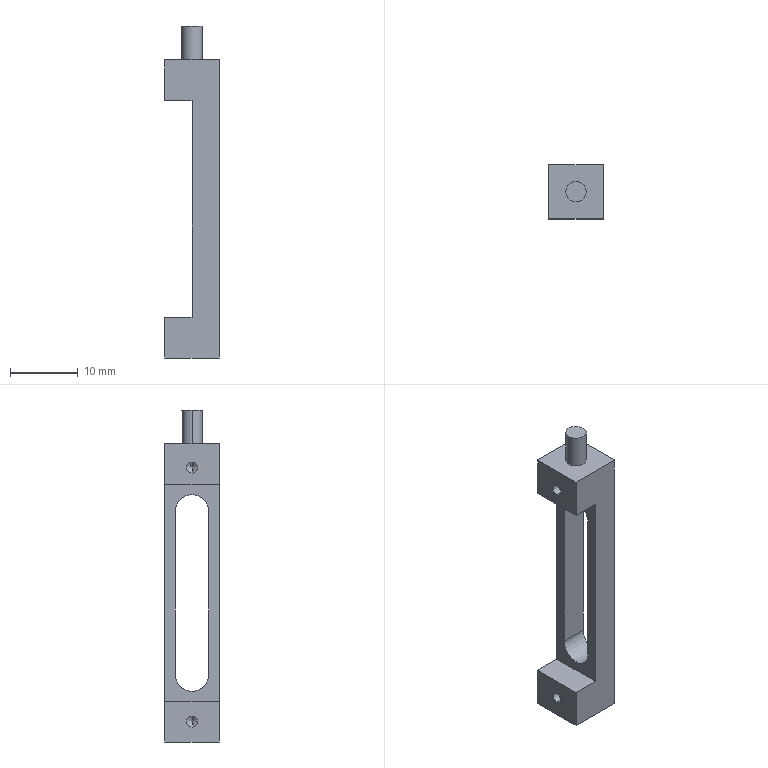Part | STEP file | 06-01-16 light source mounting plate | 1 solid | 25 faces | box 8 x 8 x 49 mm | volume 1247 mm3 | plane 13 | cylinder 8 | cone 4 | commonest cylinder face diameters 1.6 x4 3 x2 5 x2
STEP:
#1=CARTESIAN_POINT('',(1.2,0.,39.7));
#2=VERTEX_POINT('',#1);
#3=CARTESIAN_POINT('',(1.2,0.,41.3));
#4=VERTEX_POINT('',#3);
#5=CARTESIAN_POINT('',(1.2,0.,40.5));
#6=DIRECTION('',(-1.,0.,0.));
#7=DIRECTION('',(0.,0.,1.));
#8=AXIS2_PLACEMENT_3D('',#5,#6,#7);
#9=CIRCLE('',#8,0.8);
#10=EDGE_CURVE('',#2,#4,#9,.T.);
#11=ORIENTED_EDGE('',*,*,#10,.F.);
#12=CARTESIAN_POINT('',(-4.,0.,39.7));
#13=VERTEX_POINT('',#12);
#14=CARTESIAN_POINT('',(-4.,0.,39.7));
#15=DIRECTION('',(-1.,0.,0.));
#16=VECTOR('',#15,1000.);
#17=LINE('',#14,#16);
#18=EDGE_CURVE('',#2,#13,#17,.T.);
#19=ORIENTED_EDGE('',*,*,#18,.T.);
#20=CARTESIAN_POINT('',(-4.,0.,41.3));
#21=VERTEX_POINT('',#20);
#22=CARTESIAN_POINT('',(-4.,0.,40.5));
#23=DIRECTION('',(-1.,0.,0.));
#24=DIRECTION('',(0.,0.,1.));
#25=AXIS2_PLACEMENT_3D('',#22,#23,#24);
#26=CIRCLE('',#25,0.8);
#27=EDGE_CURVE('',#13,#21,#26,.T.);
#28=ORIENTED_EDGE('',*,*,#27,.T.);
#29=CARTESIAN_POINT('',(-4.,0.,41.3));
#30=DIRECTION('',(-1.,0.,0.));
#31=VECTOR('',#30,1000.);
#32=LINE('',#29,#31);
#33=EDGE_CURVE('',#4,#21,#32,.T.);
#34=ORIENTED_EDGE('',*,*,#33,.F.);
#35=EDGE_LOOP('',(#11,#19,#28,#34));
#36=FACE_OUTER_BOUND('',#35,.T.);
#37=CARTESIAN_POINT('',(-4.,0.,40.5));
#38=DIRECTION('',(-1.,0.,0.));
#39=DIRECTION('',(0.,0.,1.));
#40=AXIS2_PLACEMENT_3D('',#37,#38,#39);
#41=CYLINDRICAL_SURFACE('',#40,0.8);
#42=ADVANCED_FACE('',(#36),#41,.F.);
#43=CARTESIAN_POINT('',(1.681,0.,40.5));
#44=VERTEX_POINT('',#43);
#45=CARTESIAN_POINT('',(1.2,0.,41.3));
#46=DIRECTION('',(-0.515,0.,0.8572));
#47=VECTOR('',#46,1000.);
#48=LINE('',#45,#47);
#49=EDGE_CURVE('',#44,#4,#48,.T.);
#50=ORIENTED_EDGE('',*,*,#49,.F.);
#51=CARTESIAN_POINT('',(1.2,0.,39.7));
#52=DIRECTION('',(-0.515,0.,-0.8572));
#53=VECTOR('',#52,1000.);
#54=LINE('',#51,#53);
#55=EDGE_CURVE('',#44,#2,#54,.T.);
#56=ORIENTED_EDGE('',*,*,#55,.T.);
#57=ORIENTED_EDGE('',*,*,#10,.T.);
#58=EDGE_LOOP('',(#50,#56,#57));
#59=FACE_OUTER_BOUND('',#58,.T.);
#60=CARTESIAN_POINT('',(1.2,0.,40.5));
#61=DIRECTION('',(-1.,0.,0.));
#62=DIRECTION('',(0.,0.,1.));
#63=AXIS2_PLACEMENT_3D('',#60,#61,#62);
#64=CONICAL_SURFACE('',#63,0.8,1.03);
#65=ADVANCED_FACE('',(#59),#64,.F.);
#66=CARTESIAN_POINT('',(1.2,0.,2.2));
#67=VERTEX_POINT('',#66);
#68=CARTESIAN_POINT('',(1.2,0.,3.8));
#69=VERTEX_POINT('',#68);
#70=CARTESIAN_POINT('',(1.2,0.,3.));
#71=DIRECTION('',(-1.,0.,0.));
#72=DIRECTION('',(0.,0.,1.));
#73=AXIS2_PLACEMENT_3D('',#70,#71,#72);
#74=CIRCLE('',#73,0.8);
#75=EDGE_CURVE('',#67,#69,#74,.T.);
#76=ORIENTED_EDGE('',*,*,#75,.F.);
#77=CARTESIAN_POINT('',(-4.,0.,2.2));
#78=VERTEX_POINT('',#77);
#79=CARTESIAN_POINT('',(-4.,0.,2.2));
#80=DIRECTION('',(-1.,0.,0.));
#81=VECTOR('',#80,1000.);
#82=LINE('',#79,#81);
#83=EDGE_CURVE('',#67,#78,#82,.T.);
#84=ORIENTED_EDGE('',*,*,#83,.T.);
#85=CARTESIAN_POINT('',(-4.,0.,3.8));
#86=VERTEX_POINT('',#85);
#87=CARTESIAN_POINT('',(-4.,0.,3.));
#88=DIRECTION('',(-1.,0.,0.));
#89=DIRECTION('',(0.,0.,1.));
#90=AXIS2_PLACEMENT_3D('',#87,#88,#89);
#91=CIRCLE('',#90,0.8);
#92=EDGE_CURVE('',#78,#86,#91,.T.);
#93=ORIENTED_EDGE('',*,*,#92,.T.);
#94=CARTESIAN_POINT('',(-4.,0.,3.8));
#95=DIRECTION('',(-1.,0.,0.));
#96=VECTOR('',#95,1000.);
#97=LINE('',#94,#96);
#98=EDGE_CURVE('',#69,#86,#97,.T.);
#99=ORIENTED_EDGE('',*,*,#98,.F.);
#100=EDGE_LOOP('',(#76,#84,#93,#99));
#101=FACE_OUTER_BOUND('',#100,.T.);
#102=CARTESIAN_POINT('',(-4.,0.,3.));
#103=DIRECTION('',(-1.,0.,0.));
#104=DIRECTION('',(0.,0.,1.));
#105=AXIS2_PLACEMENT_3D('',#102,#103,#104);
#106=CYLINDRICAL_SURFACE('',#105,0.8);
#107=ADVANCED_FACE('',(#101),#106,.F.);
#108=CARTESIAN_POINT('',(1.681,0.,3.));
#109=VERTEX_POINT('',#108);
#110=CARTESIAN_POINT('',(1.2,0.,3.8));
#111=DIRECTION('',(-0.515,0.,0.8572));
#112=VECTOR('',#111,1000.);
#113=LINE('',#110,#112);
#114=EDGE_CURVE('',#109,#69,#113,.T.);
#115=ORIENTED_EDGE('',*,*,#114,.F.);
#116=CARTESIAN_POINT('',(1.2,0.,2.2));
#117=DIRECTION('',(-0.515,0.,-0.8572));
#118=VECTOR('',#117,1000.);
#119=LINE('',#116,#118);
#120=EDGE_CURVE('',#109,#67,#119,.T.);
#121=ORIENTED_EDGE('',*,*,#120,.T.);
#122=ORIENTED_EDGE('',*,*,#75,.T.);
#123=EDGE_LOOP('',(#115,#121,#122));
#124=FACE_OUTER_BOUND('',#123,.T.);
#125=CARTESIAN_POINT('',(1.2,0.,3.));
#126=DIRECTION('',(-1.,0.,0.));
#127=DIRECTION('',(0.,0.,1.));
#128=AXIS2_PLACEMENT_3D('',#125,#126,#127);
#129=CONICAL_SURFACE('',#128,0.8,1.03);
#130=ADVANCED_FACE('',(#124),#129,.F.);
#131=CARTESIAN_POINT('',(1.5,0.,49.));
#132=VERTEX_POINT('',#131);
#133=CARTESIAN_POINT('',(-1.5,0.,49.));
#134=VERTEX_POINT('',#133);
#135=CARTESIAN_POINT('',(0.,0.,49.));
#136=DIRECTION('',(0.,0.,1.));
#137=DIRECTION('',(1.,0.,0.));
#138=AXIS2_PLACEMENT_3D('',#135,#136,#137);
#139=CIRCLE('',#138,1.5);
#140=EDGE_CURVE('',#132,#134,#139,.T.);
#141=ORIENTED_EDGE('',*,*,#140,.F.);
#142=CARTESIAN_POINT('',(1.5,0.,44.));
#143=VERTEX_POINT('',#142);
#144=CARTESIAN_POINT('',(1.5,0.,49.));
#145=DIRECTION('',(0.,0.,-1.));
#146=VECTOR('',#145,1000.);
#147=LINE('',#144,#146);
#148=EDGE_CURVE('',#132,#143,#147,.T.);
#149=ORIENTED_EDGE('',*,*,#148,.T.);
#150=CARTESIAN_POINT('',(-1.5,0.,44.));
#151=VERTEX_POINT('',#150);
#152=CARTESIAN_POINT('',(0.,0.,44.));
#153=DIRECTION('',(0.,0.,1.));
#154=DIRECTION('',(1.,0.,0.));
#155=AXIS2_PLACEMENT_3D('',#152,#153,#154);
#156=CIRCLE('',#155,1.5);
#157=EDGE_CURVE('',#143,#151,#156,.T.);
#158=ORIENTED_EDGE('',*,*,#157,.T.);
#159=CARTESIAN_POINT('',(-1.5,0.,49.));
#160=DIRECTION('',(0.,0.,-1.));
#161=VECTOR('',#160,1000.);
#162=LINE('',#159,#161);
#163=EDGE_CURVE('',#134,#151,#162,.T.);
#164=ORIENTED_EDGE('',*,*,#163,.F.);
#165=EDGE_LOOP('',(#141,#149,#158,#164));
#166=FACE_OUTER_BOUND('',#165,.T.);
#167=CARTESIAN_POINT('',(0.,0.,49.));
#168=DIRECTION('',(0.,0.,-1.));
#169=DIRECTION('',(-1.,0.,0.));
#170=AXIS2_PLACEMENT_3D('',#167,#168,#169);
#171=CYLINDRICAL_SURFACE('',#170,1.5);
#172=ADVANCED_FACE('',(#166),#171,.T.);
#173=CARTESIAN_POINT('',(4.,-4.,44.));
#174=VERTEX_POINT('',#173);
#175=CARTESIAN_POINT('',(4.,4.,44.));
#176=VERTEX_POINT('',#175);
#177=CARTESIAN_POINT('',(4.,4.,44.));
#178=DIRECTION('',(0.,1.,0.));
#179=VECTOR('',#178,1000.);
#180=LINE('',#177,#179);
#181=EDGE_CURVE('',#174,#176,#180,.T.);
#182=ORIENTED_EDGE('',*,*,#181,.T.);
#183=CARTESIAN_POINT('',(-4.,4.,44.));
#184=VERTEX_POINT('',#183);
#185=CARTESIAN_POINT('',(-4.,4.,44.));
#186=DIRECTION('',(-1.,0.,0.));
#187=VECTOR('',#186,1000.);
#188=LINE('',#185,#187);
#189=EDGE_CURVE('',#176,#184,#188,.T.);
#190=ORIENTED_EDGE('',*,*,#189,.T.);
#191=CARTESIAN_POINT('',(-4.,-4.,44.));
#192=VERTEX_POINT('',#191);
#193=CARTESIAN_POINT('',(-4.,4.,44.));
#194=DIRECTION('',(0.,-1.,0.));
#195=VECTOR('',#194,1000.);
#196=LINE('',#193,#195);
#197=EDGE_CURVE('',#184,#192,#196,.T.);
#198=ORIENTED_EDGE('',*,*,#197,.T.);
#199=CARTESIAN_POINT('',(-4.,-4.,44.));
#200=DIRECTION('',(1.,0.,0.));
#201=VECTOR('',#200,1000.);
#202=LINE('',#199,#201);
#203=EDGE_CURVE('',#192,#174,#202,.T.);
#204=ORIENTED_EDGE('',*,*,#203,.T.);
#205=EDGE_LOOP('',(#182,#190,#198,#204));
#206=FACE_OUTER_BOUND('',#205,.T.);
#207=CARTESIAN_POINT('',(0.,0.,44.));
#208=DIRECTION('',(0.,0.,1.));
#209=DIRECTION('',(1.,0.,0.));
#210=AXIS2_PLACEMENT_3D('',#207,#208,#209);
#211=CIRCLE('',#210,1.5);
#212=EDGE_CURVE('',#151,#143,#211,.T.);
#213=ORIENTED_EDGE('',*,*,#212,.F.);
#214=ORIENTED_EDGE('',*,*,#157,.F.);
#215=EDGE_LOOP('',(#213,#214));
#216=FACE_BOUND('',#215,.T.);
#217=CARTESIAN_POINT('',(4.,-4.,44.));
#218=DIRECTION('',(0.,0.,1.));
#219=DIRECTION('',(1.,0.,0.));
#220=AXIS2_PLACEMENT_3D('',#217,#218,#219);
#221=PLANE('',#220);
#222=ADVANCED_FACE('',(#206,#216),#221,.T.);
#223=CARTESIAN_POINT('',(-4.,0.,40.5));
#224=DIRECTION('',(-1.,0.,0.));
#225=DIRECTION('',(0.,0.,1.));
#226=AXIS2_PLACEMENT_3D('',#223,#224,#225);
#227=CIRCLE('',#226,0.8);
#228=EDGE_CURVE('',#21,#13,#227,.T.);
#229=ORIENTED_EDGE('',*,*,#228,.F.);
#230=ORIENTED_EDGE('',*,*,#27,.F.);
#231=EDGE_LOOP('',(#229,#230));
#232=FACE_BOUND('',#231,.T.);
#233=CARTESIAN_POINT('',(-4.,4.,38.));
#234=VERTEX_POINT('',#233);
#235=CARTESIAN_POINT('',(-4.,4.,44.));
#236=DIRECTION('',(0.,0.,-1.));
#237=VECTOR('',#236,1000.);
#238=LINE('',#235,#237);
#239=EDGE_CURVE('',#184,#234,#238,.T.);
#240=ORIENTED_EDGE('',*,*,#239,.T.);
#241=CARTESIAN_POINT('',(-4.,-4.,38.));
#242=VERTEX_POINT('',#241);
#243=CARTESIAN_POINT('',(-4.,14.,38.));
#244=DIRECTION('',(0.,-1.,0.));
#245=VECTOR('',#244,1000.);
#246=LINE('',#243,#245);
#247=EDGE_CURVE('',#234,#242,#246,.T.);
#248=ORIENTED_EDGE('',*,*,#247,.T.);
#249=CARTESIAN_POINT('',(-4.,-4.,44.));
#250=DIRECTION('',(0.,0.,-1.));
#251=VECTOR('',#250,1000.);
#252=LINE('',#249,#251);
#253=EDGE_CURVE('',#192,#242,#252,.T.);
#254=ORIENTED_EDGE('',*,*,#253,.F.);
#255=ORIENTED_EDGE('',*,*,#197,.F.);
#256=EDGE_LOOP('',(#240,#248,#254,#255));
#257=FACE_OUTER_BOUND('',#256,.T.);
#258=CARTESIAN_POINT('',(-4.,4.,44.));
#259=DIRECTION('',(1.,0.,0.));
#260=DIRECTION('',(0.,1.,0.));
#261=AXIS2_PLACEMENT_3D('',#258,#259,#260);
#262=PLANE('',#261);
#263=ADVANCED_FACE('',(#232,#257),#262,.F.);
#264=CARTESIAN_POINT('',(4.,-2.5,34.));
#265=VERTEX_POINT('',#264);
#266=CARTESIAN_POINT('',(4.,-2.5,10.));
#267=VERTEX_POINT('',#266);
#268=CARTESIAN_POINT('',(4.,-2.5,34.));
#269=DIRECTION('',(0.,0.,-1.));
#270=VECTOR('',#269,1000.);
#271=LINE('',#268,#270);
#272=EDGE_CURVE('',#265,#267,#271,.T.);
#273=ORIENTED_EDGE('',*,*,#272,.F.);
#274=CARTESIAN_POINT('',(4.,2.5,34.));
#275=VERTEX_POINT('',#274);
#276=CARTESIAN_POINT('',(4.,0.,34.));
#277=DIRECTION('',(1.,0.,0.));
#278=DIRECTION('',(0.,1.,0.));
#279=AXIS2_PLACEMENT_3D('',#276,#277,#278);
#280=CIRCLE('',#279,2.5);
#281=EDGE_CURVE('',#275,#265,#280,.T.);
#282=ORIENTED_EDGE('',*,*,#281,.F.);
#283=CARTESIAN_POINT('',(4.,2.5,10.));
#284=VERTEX_POINT('',#283);
#285=CARTESIAN_POINT('',(4.,2.5,34.));
#286=DIRECTION('',(0.,0.,1.));
#287=VECTOR('',#286,1000.);
#288=LINE('',#285,#287);
#289=EDGE_CURVE('',#284,#275,#288,.T.);
#290=ORIENTED_EDGE('',*,*,#289,.F.);
#291=CARTESIAN_POINT('',(4.,0.,10.));
#292=DIRECTION('',(1.,0.,0.));
#293=DIRECTION('',(0.,1.,0.));
#294=AXIS2_PLACEMENT_3D('',#291,#292,#293);
#295=CIRCLE('',#294,2.5);
#296=EDGE_CURVE('',#267,#284,#295,.T.);
#297=ORIENTED_EDGE('',*,*,#296,.F.);
#298=EDGE_LOOP('',(#273,#282,#290,#297));
#299=FACE_BOUND('',#298,.T.);
#300=CARTESIAN_POINT('',(4.,-4.,0.));
#301=VERTEX_POINT('',#300);
#302=CARTESIAN_POINT('',(4.,4.,0.));
#303=VERTEX_POINT('',#302);
#304=CARTESIAN_POINT('',(4.,4.,0.));
#305=DIRECTION('',(0.,1.,0.));
#306=VECTOR('',#305,1000.);
#307=LINE('',#304,#306);
#308=EDGE_CURVE('',#301,#303,#307,.T.);
#309=ORIENTED_EDGE('',*,*,#308,.T.);
#310=CARTESIAN_POINT('',(4.,4.,44.));
#311=DIRECTION('',(0.,0.,-1.));
#312=VECTOR('',#311,1000.);
#313=LINE('',#310,#312);
#314=EDGE_CURVE('',#176,#303,#313,.T.);
#315=ORIENTED_EDGE('',*,*,#314,.F.);
#316=ORIENTED_EDGE('',*,*,#181,.F.);
#317=CARTESIAN_POINT('',(4.,-4.,44.));
#318=DIRECTION('',(0.,0.,-1.));
#319=VECTOR('',#318,1000.);
#320=LINE('',#317,#319);
#321=EDGE_CURVE('',#174,#301,#320,.T.);
#322=ORIENTED_EDGE('',*,*,#321,.T.);
#323=EDGE_LOOP('',(#309,#315,#316,#322));
#324=FACE_OUTER_BOUND('',#323,.T.);
#325=CARTESIAN_POINT('',(4.,4.,44.));
#326=DIRECTION('',(-1.,0.,0.));
#327=DIRECTION('',(0.,-1.,0.));
#328=AXIS2_PLACEMENT_3D('',#325,#326,#327);
#329=PLANE('',#328);
#330=ADVANCED_FACE('',(#299,#324),#329,.F.);
#331=CARTESIAN_POINT('',(0.,4.,6.));
#332=VERTEX_POINT('',#331);
#333=CARTESIAN_POINT('',(0.,4.,38.));
#334=VERTEX_POINT('',#333);
#335=CARTESIAN_POINT('',(0.,4.,44.));
#336=DIRECTION('',(0.,0.,1.));
#337=VECTOR('',#336,1000.);
#338=LINE('',#335,#337);
#339=EDGE_CURVE('',#332,#334,#338,.T.);
#340=ORIENTED_EDGE('',*,*,#339,.T.);
#341=CARTESIAN_POINT('',(-4.,4.,38.));
#342=DIRECTION('',(-1.,0.,0.));
#343=VECTOR('',#342,1000.);
#344=LINE('',#341,#343);
#345=EDGE_CURVE('',#334,#234,#344,.T.);
#346=ORIENTED_EDGE('',*,*,#345,.T.);
#347=ORIENTED_EDGE('',*,*,#239,.F.);
#348=ORIENTED_EDGE('',*,*,#189,.F.);
#349=ORIENTED_EDGE('',*,*,#314,.T.);
#350=CARTESIAN_POINT('',(-4.,4.,0.));
#351=VERTEX_POINT('',#350);
#352=CARTESIAN_POINT('',(-4.,4.,0.));
#353=DIRECTION('',(-1.,0.,0.));
#354=VECTOR('',#353,1000.);
#355=LINE('',#352,#354);
#356=EDGE_CURVE('',#303,#351,#355,.T.);
#357=ORIENTED_EDGE('',*,*,#356,.T.);
#358=CARTESIAN_POINT('',(-4.,4.,6.));
#359=VERTEX_POINT('',#358);
#360=CARTESIAN_POINT('',(-4.,4.,44.));
#361=DIRECTION('',(0.,0.,-1.));
#362=VECTOR('',#361,1000.);
#363=LINE('',#360,#362);
#364=EDGE_CURVE('',#359,#351,#363,.T.);
#365=ORIENTED_EDGE('',*,*,#364,.F.);
#366=CARTESIAN_POINT('',(-4.,4.,6.));
#367=DIRECTION('',(1.,0.,0.));
#368=VECTOR('',#367,1000.);
#369=LINE('',#366,#368);
#370=EDGE_CURVE('',#359,#332,#369,.T.);
#371=ORIENTED_EDGE('',*,*,#370,.T.);
#372=EDGE_LOOP('',(#340,#346,#347,#348,#349,#357,#365,#371));
#373=FACE_OUTER_BOUND('',#372,.T.);
#374=CARTESIAN_POINT('',(-4.,4.,44.));
#375=DIRECTION('',(0.,-1.,0.));
#376=DIRECTION('',(0.,0.,-1.));
#377=AXIS2_PLACEMENT_3D('',#374,#375,#376);
#378=PLANE('',#377);
#379=ADVANCED_FACE('',(#373),#378,.F.);
#380=CARTESIAN_POINT('',(-4.,0.,3.));
#381=DIRECTION('',(-1.,0.,0.));
#382=DIRECTION('',(0.,0.,1.));
#383=AXIS2_PLACEMENT_3D('',#380,#381,#382);
#384=CIRCLE('',#383,0.8);
#385=EDGE_CURVE('',#86,#78,#384,.T.);
#386=ORIENTED_EDGE('',*,*,#385,.F.);
#387=ORIENTED_EDGE('',*,*,#92,.F.);
#388=EDGE_LOOP('',(#386,#387));
#389=FACE_BOUND('',#388,.T.);
#390=CARTESIAN_POINT('',(-4.,-4.,6.));
#391=VERTEX_POINT('',#390);
#392=CARTESIAN_POINT('',(-4.,-4.,0.));
#393=VERTEX_POINT('',#392);
#394=CARTESIAN_POINT('',(-4.,-4.,44.));
#395=DIRECTION('',(0.,0.,-1.));
#396=VECTOR('',#395,1000.);
#397=LINE('',#394,#396);
#398=EDGE_CURVE('',#391,#393,#397,.T.);
#399=ORIENTED_EDGE('',*,*,#398,.F.);
#400=CARTESIAN_POINT('',(-4.,14.,6.));
#401=DIRECTION('',(0.,-1.,0.));
#402=VECTOR('',#401,1000.);
#403=LINE('',#400,#402);
#404=EDGE_CURVE('',#359,#391,#403,.T.);
#405=ORIENTED_EDGE('',*,*,#404,.F.);
#406=ORIENTED_EDGE('',*,*,#364,.T.);
#407=CARTESIAN_POINT('',(-4.,4.,0.));
#408=DIRECTION('',(0.,-1.,0.));
#409=VECTOR('',#408,1000.);
#410=LINE('',#407,#409);
#411=EDGE_CURVE('',#351,#393,#410,.T.);
#412=ORIENTED_EDGE('',*,*,#411,.T.);
#413=EDGE_LOOP('',(#399,#405,#406,#412));
#414=FACE_OUTER_BOUND('',#413,.T.);
#415=CARTESIAN_POINT('',(-4.,4.,44.));
#416=DIRECTION('',(1.,0.,0.));
#417=DIRECTION('',(0.,1.,0.));
#418=AXIS2_PLACEMENT_3D('',#415,#416,#417);
#419=PLANE('',#418);
#420=ADVANCED_FACE('',(#389,#414),#419,.F.);
#421=ORIENTED_EDGE('',*,*,#253,.T.);
#422=CARTESIAN_POINT('',(0.,-4.,38.));
#423=VERTEX_POINT('',#422);
#424=CARTESIAN_POINT('',(-4.,-4.,38.));
#425=DIRECTION('',(-1.,0.,0.));
#426=VECTOR('',#425,1000.);
#427=LINE('',#424,#426);
#428=EDGE_CURVE('',#423,#242,#427,.T.);
#429=ORIENTED_EDGE('',*,*,#428,.F.);
#430=CARTESIAN_POINT('',(0.,-4.,6.));
#431=VERTEX_POINT('',#430);
#432=CARTESIAN_POINT('',(0.,-4.,38.));
#433=DIRECTION('',(0.,0.,1.));
#434=VECTOR('',#433,1000.);
#435=LINE('',#432,#434);
#436=EDGE_CURVE('',#431,#423,#435,.T.);
#437=ORIENTED_EDGE('',*,*,#436,.F.);
#438=CARTESIAN_POINT('',(-4.,-4.,6.));
#439=DIRECTION('',(1.,0.,0.));
#440=VECTOR('',#439,1000.);
#441=LINE('',#438,#440);
#442=EDGE_CURVE('',#391,#431,#441,.T.);
#443=ORIENTED_EDGE('',*,*,#442,.F.);
#444=ORIENTED_EDGE('',*,*,#398,.T.);
#445=CARTESIAN_POINT('',(-4.,-4.,0.));
#446=DIRECTION('',(1.,0.,0.));
#447=VECTOR('',#446,1000.);
#448=LINE('',#445,#447);
#449=EDGE_CURVE('',#393,#301,#448,.T.);
#450=ORIENTED_EDGE('',*,*,#449,.T.);
#451=ORIENTED_EDGE('',*,*,#321,.F.);
#452=ORIENTED_EDGE('',*,*,#203,.F.);
#453=EDGE_LOOP('',(#421,#429,#437,#443,#444,#450,#451,#452));
#454=FACE_OUTER_BOUND('',#453,.T.);
#455=CARTESIAN_POINT('',(-4.,-4.,44.));
#456=DIRECTION('',(0.,1.,0.));
#457=DIRECTION('',(0.,0.,1.));
#458=AXIS2_PLACEMENT_3D('',#455,#456,#457);
#459=PLANE('',#458);
#460=ADVANCED_FACE('',(#454),#459,.F.);
#461=ORIENTED_EDGE('',*,*,#308,.F.);
#462=ORIENTED_EDGE('',*,*,#449,.F.);
#463=ORIENTED_EDGE('',*,*,#411,.F.);
#464=ORIENTED_EDGE('',*,*,#356,.F.);
#465=EDGE_LOOP('',(#461,#462,#463,#464));
#466=FACE_OUTER_BOUND('',#465,.T.);
#467=CARTESIAN_POINT('',(4.,-4.,0.));
#468=DIRECTION('',(0.,0.,1.));
#469=DIRECTION('',(1.,0.,0.));
#470=AXIS2_PLACEMENT_3D('',#467,#468,#469);
#471=PLANE('',#470);
#472=ADVANCED_FACE('',(#466),#471,.F.);
#473=CARTESIAN_POINT('',(0.,14.,38.));
#474=DIRECTION('',(0.,-1.,0.));
#475=VECTOR('',#474,1000.);
#476=LINE('',#473,#475);
#477=EDGE_CURVE('',#334,#423,#476,.T.);
#478=ORIENTED_EDGE('',*,*,#477,.T.);
#479=ORIENTED_EDGE('',*,*,#428,.T.);
#480=ORIENTED_EDGE('',*,*,#247,.F.);
#481=ORIENTED_EDGE('',*,*,#345,.F.);
#482=EDGE_LOOP('',(#478,#479,#480,#481));
#483=FACE_OUTER_BOUND('',#482,.T.);
#484=CARTESIAN_POINT('',(-4.,14.,38.));
#485=DIRECTION('',(0.,0.,1.));
#486=DIRECTION('',(1.,0.,0.));
#487=AXIS2_PLACEMENT_3D('',#484,#485,#486);
#488=PLANE('',#487);
#489=ADVANCED_FACE('',(#483),#488,.F.);
#490=CARTESIAN_POINT('',(0.,2.5,10.));
#491=VERTEX_POINT('',#490);
#492=CARTESIAN_POINT('',(0.,2.5,34.));
#493=VERTEX_POINT('',#492);
#494=CARTESIAN_POINT('',(0.,2.5,38.));
#495=DIRECTION('',(0.,0.,1.));
#496=VECTOR('',#495,1000.);
#497=LINE('',#494,#496);
#498=EDGE_CURVE('',#491,#493,#497,.T.);
#499=ORIENTED_EDGE('',*,*,#498,.T.);
#500=CARTESIAN_POINT('',(0.,-2.5,34.));
#501=VERTEX_POINT('',#500);
#502=CARTESIAN_POINT('',(0.,0.,34.));
#503=DIRECTION('',(1.,0.,0.));
#504=DIRECTION('',(0.,0.,-1.));
#505=AXIS2_PLACEMENT_3D('',#502,#503,#504);
#506=CIRCLE('',#505,2.5);
#507=EDGE_CURVE('',#493,#501,#506,.T.);
#508=ORIENTED_EDGE('',*,*,#507,.T.);
#509=CARTESIAN_POINT('',(0.,-2.5,10.));
#510=VERTEX_POINT('',#509);
#511=CARTESIAN_POINT('',(0.,-2.5,38.));
#512=DIRECTION('',(0.,0.,-1.));
#513=VECTOR('',#512,1000.);
#514=LINE('',#511,#513);
#515=EDGE_CURVE('',#501,#510,#514,.T.);
#516=ORIENTED_EDGE('',*,*,#515,.T.);
#517=CARTESIAN_POINT('',(0.,0.,10.));
#518=DIRECTION('',(1.,0.,0.));
#519=DIRECTION('',(0.,0.,-1.));
#520=AXIS2_PLACEMENT_3D('',#517,#518,#519);
#521=CIRCLE('',#520,2.5);
#522=EDGE_CURVE('',#510,#491,#521,.T.);
#523=ORIENTED_EDGE('',*,*,#522,.T.);
#524=EDGE_LOOP('',(#499,#508,#516,#523));
#525=FACE_BOUND('',#524,.T.);
#526=CARTESIAN_POINT('',(0.,14.,6.));
#527=DIRECTION('',(0.,-1.,0.));
#528=VECTOR('',#527,1000.);
#529=LINE('',#526,#528);
#530=EDGE_CURVE('',#332,#431,#529,.T.);
#531=ORIENTED_EDGE('',*,*,#530,.T.);
#532=ORIENTED_EDGE('',*,*,#436,.T.);
#533=ORIENTED_EDGE('',*,*,#477,.F.);
#534=ORIENTED_EDGE('',*,*,#339,.F.);
#535=EDGE_LOOP('',(#531,#532,#533,#534));
#536=FACE_OUTER_BOUND('',#535,.T.);
#537=CARTESIAN_POINT('',(0.,14.,38.));
#538=DIRECTION('',(1.,0.,0.));
#539=DIRECTION('',(0.,0.,-1.));
#540=AXIS2_PLACEMENT_3D('',#537,#538,#539);
#541=PLANE('',#540);
#542=ADVANCED_FACE('',(#525,#536),#541,.F.);
#543=ORIENTED_EDGE('',*,*,#404,.T.);
#544=ORIENTED_EDGE('',*,*,#442,.T.);
#545=ORIENTED_EDGE('',*,*,#530,.F.);
#546=ORIENTED_EDGE('',*,*,#370,.F.);
#547=EDGE_LOOP('',(#543,#544,#545,#546));
#548=FACE_OUTER_BOUND('',#547,.T.);
#549=CARTESIAN_POINT('',(-4.,14.,6.));
#550=DIRECTION('',(0.,0.,-1.));
#551=DIRECTION('',(-1.,0.,0.));
#552=AXIS2_PLACEMENT_3D('',#549,#550,#551);
#553=PLANE('',#552);
#554=ADVANCED_FACE('',(#548),#553,.F.);
#555=CARTESIAN_POINT('',(-6.,2.5,34.));
#556=DIRECTION('',(1.,0.,0.));
#557=VECTOR('',#556,1000.);
#558=LINE('',#555,#557);
#559=EDGE_CURVE('',#493,#275,#558,.T.);
#560=ORIENTED_EDGE('',*,*,#559,.T.);
#561=ORIENTED_EDGE('',*,*,#281,.T.);
#562=CARTESIAN_POINT('',(-6.,-2.5,34.));
#563=DIRECTION('',(1.,0.,0.));
#564=VECTOR('',#563,1000.);
#565=LINE('',#562,#564);
#566=EDGE_CURVE('',#501,#265,#565,.T.);
#567=ORIENTED_EDGE('',*,*,#566,.F.);
#568=ORIENTED_EDGE('',*,*,#507,.F.);
#569=EDGE_LOOP('',(#560,#561,#567,#568));
#570=FACE_OUTER_BOUND('',#569,.T.);
#571=CARTESIAN_POINT('',(-6.,0.,34.));
#572=DIRECTION('',(1.,0.,0.));
#573=DIRECTION('',(0.,1.,0.));
#574=AXIS2_PLACEMENT_3D('',#571,#572,#573);
#575=CYLINDRICAL_SURFACE('',#574,2.5);
#576=ADVANCED_FACE('',(#570),#575,.F.);
#577=CARTESIAN_POINT('',(-6.,2.5,10.));
#578=DIRECTION('',(1.,0.,0.));
#579=VECTOR('',#578,1000.);
#580=LINE('',#577,#579);
#581=EDGE_CURVE('',#491,#284,#580,.T.);
#582=ORIENTED_EDGE('',*,*,#581,.T.);
#583=ORIENTED_EDGE('',*,*,#289,.T.);
#584=ORIENTED_EDGE('',*,*,#559,.F.);
#585=ORIENTED_EDGE('',*,*,#498,.F.);
#586=EDGE_LOOP('',(#582,#583,#584,#585));
#587=FACE_OUTER_BOUND('',#586,.T.);
#588=CARTESIAN_POINT('',(-6.,2.5,34.));
#589=DIRECTION('',(0.,1.,0.));
#590=DIRECTION('',(-1.,0.,0.));
#591=AXIS2_PLACEMENT_3D('',#588,#589,#590);
#592=PLANE('',#591);
#593=ADVANCED_FACE('',(#587),#592,.F.);
#594=CARTESIAN_POINT('',(-6.,-2.5,10.));
#595=DIRECTION('',(1.,0.,0.));
#596=VECTOR('',#595,1000.);
#597=LINE('',#594,#596);
#598=EDGE_CURVE('',#510,#267,#597,.T.);
#599=ORIENTED_EDGE('',*,*,#598,.T.);
#600=ORIENTED_EDGE('',*,*,#296,.T.);
#601=ORIENTED_EDGE('',*,*,#581,.F.);
#602=ORIENTED_EDGE('',*,*,#522,.F.);
#603=EDGE_LOOP('',(#599,#600,#601,#602));
#604=FACE_OUTER_BOUND('',#603,.T.);
#605=CARTESIAN_POINT('',(-6.,0.,10.));
#606=DIRECTION('',(1.,0.,0.));
#607=DIRECTION('',(0.,1.,0.));
#608=AXIS2_PLACEMENT_3D('',#605,#606,#607);
#609=CYLINDRICAL_SURFACE('',#608,2.5);
#610=ADVANCED_FACE('',(#604),#609,.F.);
#611=ORIENTED_EDGE('',*,*,#566,.T.);
#612=ORIENTED_EDGE('',*,*,#272,.T.);
#613=ORIENTED_EDGE('',*,*,#598,.F.);
#614=ORIENTED_EDGE('',*,*,#515,.F.);
#615=EDGE_LOOP('',(#611,#612,#613,#614));
#616=FACE_OUTER_BOUND('',#615,.T.);
#617=CARTESIAN_POINT('',(-6.,-2.5,34.));
#618=DIRECTION('',(0.,-1.,0.));
#619=DIRECTION('',(1.,0.,0.));
#620=AXIS2_PLACEMENT_3D('',#617,#618,#619);
#621=PLANE('',#620);
#622=ADVANCED_FACE('',(#616),#621,.F.);
#623=ORIENTED_EDGE('',*,*,#148,.F.);
#624=CARTESIAN_POINT('',(0.,0.,49.));
#625=DIRECTION('',(0.,0.,1.));
#626=DIRECTION('',(1.,0.,0.));
#627=AXIS2_PLACEMENT_3D('',#624,#625,#626);
#628=CIRCLE('',#627,1.5);
#629=EDGE_CURVE('',#134,#132,#628,.T.);
#630=ORIENTED_EDGE('',*,*,#629,.F.);
#631=ORIENTED_EDGE('',*,*,#163,.T.);
#632=ORIENTED_EDGE('',*,*,#212,.T.);
#633=EDGE_LOOP('',(#623,#630,#631,#632));
#634=FACE_OUTER_BOUND('',#633,.T.);
#635=CARTESIAN_POINT('',(0.,0.,49.));
#636=DIRECTION('',(0.,0.,-1.));
#637=DIRECTION('',(-1.,0.,0.));
#638=AXIS2_PLACEMENT_3D('',#635,#636,#637);
#639=CYLINDRICAL_SURFACE('',#638,1.5);
#640=ADVANCED_FACE('',(#634),#639,.T.);
#641=ORIENTED_EDGE('',*,*,#629,.T.);
#642=ORIENTED_EDGE('',*,*,#140,.T.);
#643=EDGE_LOOP('',(#641,#642));
#644=FACE_OUTER_BOUND('',#643,.T.);
#645=CARTESIAN_POINT('',(0.,0.,49.));
#646=DIRECTION('',(0.,0.,1.));
#647=DIRECTION('',(1.,0.,0.));
#648=AXIS2_PLACEMENT_3D('',#645,#646,#647);
#649=PLANE('',#648);
#650=ADVANCED_FACE('',(#644),#649,.T.);
#651=ORIENTED_EDGE('',*,*,#120,.F.);
#652=ORIENTED_EDGE('',*,*,#114,.T.);
#653=CARTESIAN_POINT('',(1.2,0.,3.));
#654=DIRECTION('',(-1.,0.,0.));
#655=DIRECTION('',(0.,0.,1.));
#656=AXIS2_PLACEMENT_3D('',#653,#654,#655);
#657=CIRCLE('',#656,0.8);
#658=EDGE_CURVE('',#69,#67,#657,.T.);
#659=ORIENTED_EDGE('',*,*,#658,.T.);
#660=EDGE_LOOP('',(#651,#652,#659));
#661=FACE_OUTER_BOUND('',#660,.T.);
#662=CARTESIAN_POINT('',(1.2,0.,3.));
#663=DIRECTION('',(-1.,0.,0.));
#664=DIRECTION('',(0.,0.,1.));
#665=AXIS2_PLACEMENT_3D('',#662,#663,#664);
#666=CONICAL_SURFACE('',#665,0.8,1.03);
#667=ADVANCED_FACE('',(#661),#666,.F.);
#668=ORIENTED_EDGE('',*,*,#83,.F.);
#669=ORIENTED_EDGE('',*,*,#658,.F.);
#670=ORIENTED_EDGE('',*,*,#98,.T.);
#671=ORIENTED_EDGE('',*,*,#385,.T.);
#672=EDGE_LOOP('',(#668,#669,#670,#671));
#673=FACE_OUTER_BOUND('',#672,.T.);
#674=CARTESIAN_POINT('',(-4.,0.,3.));
#675=DIRECTION('',(-1.,0.,0.));
#676=DIRECTION('',(0.,0.,1.));
#677=AXIS2_PLACEMENT_3D('',#674,#675,#676);
#678=CYLINDRICAL_SURFACE('',#677,0.8);
#679=ADVANCED_FACE('',(#673),#678,.F.);
#680=ORIENTED_EDGE('',*,*,#55,.F.);
#681=ORIENTED_EDGE('',*,*,#49,.T.);
#682=CARTESIAN_POINT('',(1.2,0.,40.5));
#683=DIRECTION('',(-1.,0.,0.));
#684=DIRECTION('',(0.,0.,1.));
#685=AXIS2_PLACEMENT_3D('',#682,#683,#684);
#686=CIRCLE('',#685,0.8);
#687=EDGE_CURVE('',#4,#2,#686,.T.);
#688=ORIENTED_EDGE('',*,*,#687,.T.);
#689=EDGE_LOOP('',(#680,#681,#688));
#690=FACE_OUTER_BOUND('',#689,.T.);
#691=CARTESIAN_POINT('',(1.2,0.,40.5));
#692=DIRECTION('',(-1.,0.,0.));
#693=DIRECTION('',(0.,0.,1.));
#694=AXIS2_PLACEMENT_3D('',#691,#692,#693);
#695=CONICAL_SURFACE('',#694,0.8,1.03);
#696=ADVANCED_FACE('',(#690),#695,.F.);
#697=ORIENTED_EDGE('',*,*,#18,.F.);
#698=ORIENTED_EDGE('',*,*,#687,.F.);
#699=ORIENTED_EDGE('',*,*,#33,.T.);
#700=ORIENTED_EDGE('',*,*,#228,.T.);
#701=EDGE_LOOP('',(#697,#698,#699,#700));
#702=FACE_OUTER_BOUND('',#701,.T.);
#703=CARTESIAN_POINT('',(-4.,0.,40.5));
#704=DIRECTION('',(-1.,0.,0.));
#705=DIRECTION('',(0.,0.,1.));
#706=AXIS2_PLACEMENT_3D('',#703,#704,#705);
#707=CYLINDRICAL_SURFACE('',#706,0.8);
#708=ADVANCED_FACE('',(#702),#707,.F.);
#709=CLOSED_SHELL('',(#42,#65,#107,#130,#172,#222,#263,#330,#379,#420,#460,#472,#489,#542,#554,#576,#593,#610,#622,#640,#650,#667,#679,#696,#708));
#710=MANIFOLD_SOLID_BREP('',#709);
#711=CARTESIAN_POINT('',(0.,0.,0.));
#712=DIRECTION('',(0.,0.,1.));
#713=DIRECTION('',(1.,0.,0.));
#714=AXIS2_PLACEMENT_3D('',#711,#712,#713);
#715=(LENGTH_UNIT()NAMED_UNIT(*)SI_UNIT(.MILLI.,.METRE.));
#716=UNCERTAINTY_MEASURE_WITH_UNIT(LENGTH_MEASURE(0.00001),#715,'','');
#717=(NAMED_UNIT(*)PLANE_ANGLE_UNIT()SI_UNIT($,.RADIAN.));
#718=(NAMED_UNIT(*)SI_UNIT($,.STERADIAN.)SOLID_ANGLE_UNIT());
#719=(GEOMETRIC_REPRESENTATION_CONTEXT(3)GLOBAL_UNCERTAINTY_ASSIGNED_CONTEXT((#716))GLOBAL_UNIT_ASSIGNED_CONTEXT((#715,#717,#718))REPRESENTATION_CONTEXT('',''));
#720=ADVANCED_BREP_SHAPE_REPRESENTATION('',(#710,#714),#719);